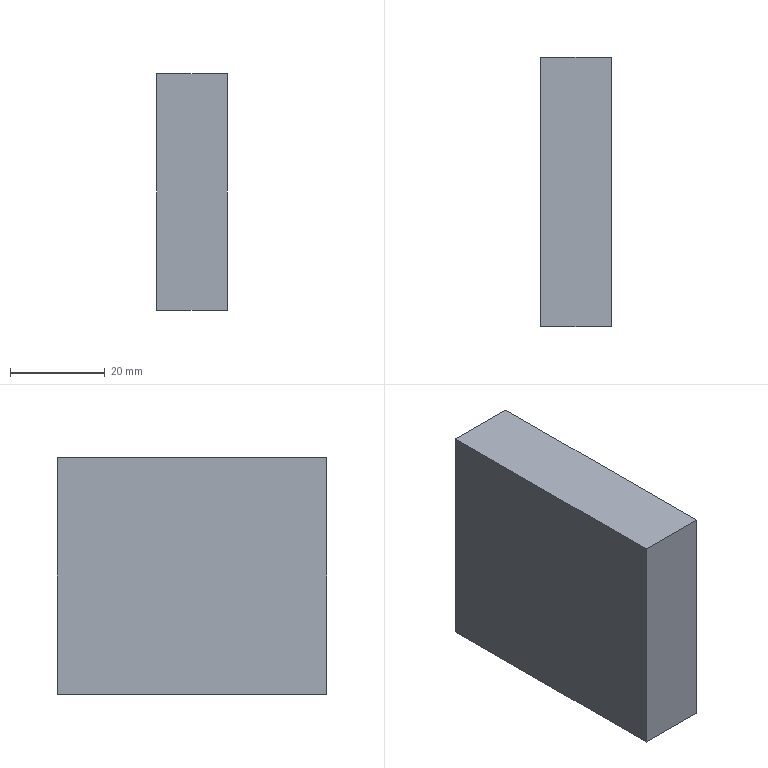Part | STEP file | Vibrator coil left support_default | 1 solid | 18 faces | box 15 x 57 x 50 mm | volume 41837 mm3 | cylinder 6 | cone 6 | plane 6 | commonest cylinder face diameters 5 x6
STEP:
#1=CARTESIAN_POINT('',(0.,0.,0.));
#2=DIRECTION('',(0.,0.,1.));
#3=DIRECTION('',(1.,0.,0.));
#4=AXIS2_PLACEMENT_3D('',#1,#2,#3);
#5=CARTESIAN_POINT('',(-2.5,-17.5,-10.));
#6=VERTEX_POINT('',#5);
#7=CARTESIAN_POINT('',(-2.5,-17.5,-25.));
#8=VERTEX_POINT('',#7);
#9=CARTESIAN_POINT('',(-2.5,-17.5,-25.));
#10=DIRECTION('',(0.,0.,-1.));
#11=VECTOR('',#10,1.);
#12=LINE('',#9,#11);
#13=CARTESIAN_POINT('',(0.,-17.5,-25.));
#14=DIRECTION('',(0.,0.,-1.));
#15=DIRECTION('',(-1.,0.,0.));
#16=AXIS2_PLACEMENT_3D('',#13,#14,#15);
#17=CYLINDRICAL_SURFACE('',#16,2.5);
#18=CARTESIAN_POINT('',(6.283,0.));
#19=DIRECTION('',(0.,1.));
#20=VECTOR('',#19,1.);
#21=LINE('',#18,#20);
#22=(GEOMETRIC_REPRESENTATION_CONTEXT(2)PARAMETRIC_REPRESENTATION_CONTEXT()REPRESENTATION_CONTEXT('',''));
#23=DEFINITIONAL_REPRESENTATION('',(#21),#22);
#24=PCURVE('',#17,#23);
#25=CARTESIAN_POINT('',(0.,-17.5,-25.));
#26=DIRECTION('',(0.,0.,-1.));
#27=DIRECTION('',(-1.,0.,0.));
#28=AXIS2_PLACEMENT_3D('',#25,#26,#27);
#29=CYLINDRICAL_SURFACE('',#28,2.5);
#30=CARTESIAN_POINT('',(0.,0.));
#31=DIRECTION('',(0.,1.));
#32=VECTOR('',#31,1.);
#33=LINE('',#30,#32);
#34=(GEOMETRIC_REPRESENTATION_CONTEXT(2)PARAMETRIC_REPRESENTATION_CONTEXT()REPRESENTATION_CONTEXT('',''));
#35=DEFINITIONAL_REPRESENTATION('',(#33),#34);
#36=PCURVE('',#29,#35);
#37=SURFACE_CURVE('',#12,(#24,#36),.PCURVE_S1.);
#38=EDGE_CURVE('',#6,#8,#37,.T.);
#39=ORIENTED_EDGE('',*,*,#38,.T.);
#40=CARTESIAN_POINT('',(2.5,-17.5,-25.));
#41=VERTEX_POINT('',#40);
#42=CARTESIAN_POINT('',(0.,-17.5,-25.));
#43=DIRECTION('',(0.,0.,-1.));
#44=DIRECTION('',(-1.,0.,0.));
#45=AXIS2_PLACEMENT_3D('',#42,#43,#44);
#46=CIRCLE('',#45,2.5);
#47=CARTESIAN_POINT('',(0.,0.));
#48=DIRECTION('',(1.,0.));
#49=VECTOR('',#48,1.);
#50=LINE('',#47,#49);
#51=(GEOMETRIC_REPRESENTATION_CONTEXT(2)PARAMETRIC_REPRESENTATION_CONTEXT()REPRESENTATION_CONTEXT('',''));
#52=DEFINITIONAL_REPRESENTATION('',(#50),#51);
#53=PCURVE('',#17,#52);
#54=CARTESIAN_POINT('',(0.,0.,-25.));
#55=DIRECTION('',(0.,0.,1.));
#56=DIRECTION('',(1.,0.,0.));
#57=AXIS2_PLACEMENT_3D('',#54,#55,#56);
#58=PLANE('',#57);
#59=CARTESIAN_POINT('',(-2.5,-17.5));
#60=CARTESIAN_POINT('',(-2.5,-13.17));
#61=CARTESIAN_POINT('',(1.25,-15.335));
#62=CARTESIAN_POINT('',(5.,-17.5));
#63=CARTESIAN_POINT('',(1.25,-19.665));
#64=CARTESIAN_POINT('',(-2.5,-21.83));
#65=CARTESIAN_POINT('',(-2.5,-17.5));
#66=(BOUNDED_CURVE()B_SPLINE_CURVE(2,(#59,#60,#61,#62,#63,#64,#65),.UNSPECIFIED.,.T.,.F.)B_SPLINE_CURVE_WITH_KNOTS((1,2,2,2,2,1),(-2.094,0.,2.094,4.189,6.283,8.378),.UNSPECIFIED.)CURVE()GEOMETRIC_REPRESENTATION_ITEM()RATIONAL_B_SPLINE_CURVE((1.,0.5,1.,0.5,1.,0.5,1.))REPRESENTATION_ITEM(''));
#67=(GEOMETRIC_REPRESENTATION_CONTEXT(2)PARAMETRIC_REPRESENTATION_CONTEXT()REPRESENTATION_CONTEXT('',''));
#68=DEFINITIONAL_REPRESENTATION('',(#66),#67);
#69=PCURVE('',#58,#68);
#70=SURFACE_CURVE('',#46,(#53,#69),.PCURVE_S1.);
#71=EDGE_CURVE('',#41,#8,#70,.T.);
#72=ORIENTED_EDGE('',*,*,#71,.F.);
#73=CARTESIAN_POINT('',(2.5,-17.5,-10.));
#74=VERTEX_POINT('',#73);
#75=CARTESIAN_POINT('',(2.5,-17.5,-25.));
#76=DIRECTION('',(0.,0.,-1.));
#77=VECTOR('',#76,1.);
#78=LINE('',#75,#77);
#79=CARTESIAN_POINT('',(3.142,0.));
#80=DIRECTION('',(0.,1.));
#81=VECTOR('',#80,1.);
#82=LINE('',#79,#81);
#83=(GEOMETRIC_REPRESENTATION_CONTEXT(2)PARAMETRIC_REPRESENTATION_CONTEXT()REPRESENTATION_CONTEXT('',''));
#84=DEFINITIONAL_REPRESENTATION('',(#82),#83);
#85=PCURVE('',#17,#84);
#86=CARTESIAN_POINT('',(3.142,0.));
#87=DIRECTION('',(0.,1.));
#88=VECTOR('',#87,1.);
#89=LINE('',#86,#88);
#90=(GEOMETRIC_REPRESENTATION_CONTEXT(2)PARAMETRIC_REPRESENTATION_CONTEXT()REPRESENTATION_CONTEXT('',''));
#91=DEFINITIONAL_REPRESENTATION('',(#89),#90);
#92=PCURVE('',#29,#91);
#93=SURFACE_CURVE('',#78,(#85,#92),.PCURVE_S1.);
#94=EDGE_CURVE('',#74,#41,#93,.T.);
#95=ORIENTED_EDGE('',*,*,#94,.F.);
#96=CARTESIAN_POINT('',(0.,-17.5,-10.));
#97=DIRECTION('',(0.,0.,-1.));
#98=DIRECTION('',(-1.,0.,0.));
#99=AXIS2_PLACEMENT_3D('',#96,#97,#98);
#100=CIRCLE('',#99,2.5);
#101=CARTESIAN_POINT('',(0.,-15.));
#102=DIRECTION('',(1.,0.));
#103=VECTOR('',#102,1.);
#104=LINE('',#101,#103);
#105=(GEOMETRIC_REPRESENTATION_CONTEXT(2)PARAMETRIC_REPRESENTATION_CONTEXT()REPRESENTATION_CONTEXT('',''));
#106=DEFINITIONAL_REPRESENTATION('',(#104),#105);
#107=PCURVE('',#17,#106);
#108=CARTESIAN_POINT('',(0.,-17.5,-10.));
#109=DIRECTION('',(0.,0.,-1.));
#110=DIRECTION('',(-1.,0.,0.));
#111=AXIS2_PLACEMENT_3D('',#108,#109,#110);
#112=CONICAL_SURFACE('',#111,2.5,1.03);
#113=CARTESIAN_POINT('',(0.,0.));
#114=DIRECTION('',(1.,0.));
#115=VECTOR('',#114,1.);
#116=LINE('',#113,#115);
#117=(GEOMETRIC_REPRESENTATION_CONTEXT(2)PARAMETRIC_REPRESENTATION_CONTEXT()REPRESENTATION_CONTEXT('',''));
#118=DEFINITIONAL_REPRESENTATION('',(#116),#117);
#119=PCURVE('',#112,#118);
#120=SURFACE_CURVE('',#100,(#107,#119),.PCURVE_S1.);
#121=EDGE_CURVE('',#74,#6,#120,.T.);
#122=ORIENTED_EDGE('',*,*,#121,.T.);
#123=EDGE_LOOP('',(#39,#72,#95,#122));
#124=FACE_BOUND('',#123,.F.);
#125=ADVANCED_FACE('',(#124),#17,.F.);
#126=ORIENTED_EDGE('',*,*,#121,.F.);
#127=CARTESIAN_POINT('',(0.,-17.5,-8.498));
#128=VERTEX_POINT('',#127);
#129=CARTESIAN_POINT('',(2.5,-17.5,-10.));
#130=DIRECTION('',(0.8572,0.,-0.515));
#131=VECTOR('',#130,1.);
#132=LINE('',#129,#131);
#133=CARTESIAN_POINT('',(3.142,0.));
#134=DIRECTION('',(0.,1.));
#135=VECTOR('',#134,1.);
#136=LINE('',#133,#135);
#137=(GEOMETRIC_REPRESENTATION_CONTEXT(2)PARAMETRIC_REPRESENTATION_CONTEXT()REPRESENTATION_CONTEXT('',''));
#138=DEFINITIONAL_REPRESENTATION('',(#136),#137);
#139=PCURVE('',#112,#138);
#140=CARTESIAN_POINT('',(0.,-17.5,-10.));
#141=DIRECTION('',(0.,0.,-1.));
#142=DIRECTION('',(-1.,0.,0.));
#143=AXIS2_PLACEMENT_3D('',#140,#141,#142);
#144=CONICAL_SURFACE('',#143,2.5,1.03);
#145=CARTESIAN_POINT('',(3.142,0.));
#146=DIRECTION('',(0.,1.));
#147=VECTOR('',#146,1.);
#148=LINE('',#145,#147);
#149=(GEOMETRIC_REPRESENTATION_CONTEXT(2)PARAMETRIC_REPRESENTATION_CONTEXT()REPRESENTATION_CONTEXT('',''));
#150=DEFINITIONAL_REPRESENTATION('',(#148),#149);
#151=PCURVE('',#144,#150);
#152=SURFACE_CURVE('',#132,(#139,#151),.PCURVE_S1.);
#153=EDGE_CURVE('',#128,#74,#152,.T.);
#154=ORIENTED_EDGE('',*,*,#153,.F.);
#155=CARTESIAN_POINT('',(-2.5,-17.5,-10.));
#156=DIRECTION('',(-0.8572,0.,-0.515));
#157=VECTOR('',#156,1.);
#158=LINE('',#155,#157);
#159=CARTESIAN_POINT('',(6.283,0.));
#160=DIRECTION('',(0.,1.));
#161=VECTOR('',#160,1.);
#162=LINE('',#159,#161);
#163=(GEOMETRIC_REPRESENTATION_CONTEXT(2)PARAMETRIC_REPRESENTATION_CONTEXT()REPRESENTATION_CONTEXT('',''));
#164=DEFINITIONAL_REPRESENTATION('',(#162),#163);
#165=PCURVE('',#112,#164);
#166=CARTESIAN_POINT('',(0.,0.));
#167=DIRECTION('',(0.,1.));
#168=VECTOR('',#167,1.);
#169=LINE('',#166,#168);
#170=(GEOMETRIC_REPRESENTATION_CONTEXT(2)PARAMETRIC_REPRESENTATION_CONTEXT()REPRESENTATION_CONTEXT('',''));
#171=DEFINITIONAL_REPRESENTATION('',(#169),#170);
#172=PCURVE('',#144,#171);
#173=SURFACE_CURVE('',#158,(#165,#172),.PCURVE_S1.);
#174=EDGE_CURVE('',#128,#6,#173,.T.);
#175=ORIENTED_EDGE('',*,*,#174,.T.);
#176=EDGE_LOOP('',(#126,#154,#175));
#177=FACE_BOUND('',#176,.F.);
#178=ADVANCED_FACE('',(#177),#112,.F.);
#179=CARTESIAN_POINT('',(-2.5,17.5,-10.));
#180=VERTEX_POINT('',#179);
#181=CARTESIAN_POINT('',(-2.5,17.5,-25.));
#182=VERTEX_POINT('',#181);
#183=CARTESIAN_POINT('',(-2.5,17.5,-25.));
#184=DIRECTION('',(0.,0.,-1.));
#185=VECTOR('',#184,1.);
#186=LINE('',#183,#185);
#187=CARTESIAN_POINT('',(0.,17.5,-25.));
#188=DIRECTION('',(0.,0.,-1.));
#189=DIRECTION('',(-1.,0.,0.));
#190=AXIS2_PLACEMENT_3D('',#187,#188,#189);
#191=CYLINDRICAL_SURFACE('',#190,2.5);
#192=CARTESIAN_POINT('',(6.283,0.));
#193=DIRECTION('',(0.,1.));
#194=VECTOR('',#193,1.);
#195=LINE('',#192,#194);
#196=(GEOMETRIC_REPRESENTATION_CONTEXT(2)PARAMETRIC_REPRESENTATION_CONTEXT()REPRESENTATION_CONTEXT('',''));
#197=DEFINITIONAL_REPRESENTATION('',(#195),#196);
#198=PCURVE('',#191,#197);
#199=CARTESIAN_POINT('',(0.,17.5,-25.));
#200=DIRECTION('',(0.,0.,-1.));
#201=DIRECTION('',(-1.,0.,0.));
#202=AXIS2_PLACEMENT_3D('',#199,#200,#201);
#203=CYLINDRICAL_SURFACE('',#202,2.5);
#204=CARTESIAN_POINT('',(0.,0.));
#205=DIRECTION('',(0.,1.));
#206=VECTOR('',#205,1.);
#207=LINE('',#204,#206);
#208=(GEOMETRIC_REPRESENTATION_CONTEXT(2)PARAMETRIC_REPRESENTATION_CONTEXT()REPRESENTATION_CONTEXT('',''));
#209=DEFINITIONAL_REPRESENTATION('',(#207),#208);
#210=PCURVE('',#203,#209);
#211=SURFACE_CURVE('',#186,(#198,#210),.PCURVE_S1.);
#212=EDGE_CURVE('',#180,#182,#211,.T.);
#213=ORIENTED_EDGE('',*,*,#212,.T.);
#214=CARTESIAN_POINT('',(2.5,17.5,-25.));
#215=VERTEX_POINT('',#214);
#216=CARTESIAN_POINT('',(0.,17.5,-25.));
#217=DIRECTION('',(0.,0.,-1.));
#218=DIRECTION('',(-1.,0.,0.));
#219=AXIS2_PLACEMENT_3D('',#216,#217,#218);
#220=CIRCLE('',#219,2.5);
#221=CARTESIAN_POINT('',(0.,0.));
#222=DIRECTION('',(1.,0.));
#223=VECTOR('',#222,1.);
#224=LINE('',#221,#223);
#225=(GEOMETRIC_REPRESENTATION_CONTEXT(2)PARAMETRIC_REPRESENTATION_CONTEXT()REPRESENTATION_CONTEXT('',''));
#226=DEFINITIONAL_REPRESENTATION('',(#224),#225);
#227=PCURVE('',#191,#226);
#228=CARTESIAN_POINT('',(-2.5,17.5));
#229=CARTESIAN_POINT('',(-2.5,21.83));
#230=CARTESIAN_POINT('',(1.25,19.665));
#231=CARTESIAN_POINT('',(5.,17.5));
#232=CARTESIAN_POINT('',(1.25,15.335));
#233=CARTESIAN_POINT('',(-2.5,13.17));
#234=CARTESIAN_POINT('',(-2.5,17.5));
#235=(BOUNDED_CURVE()B_SPLINE_CURVE(2,(#228,#229,#230,#231,#232,#233,#234),.UNSPECIFIED.,.T.,.F.)B_SPLINE_CURVE_WITH_KNOTS((1,2,2,2,2,1),(-2.094,0.,2.094,4.189,6.283,8.378),.UNSPECIFIED.)CURVE()GEOMETRIC_REPRESENTATION_ITEM()RATIONAL_B_SPLINE_CURVE((1.,0.5,1.,0.5,1.,0.5,1.))REPRESENTATION_ITEM(''));
#236=(GEOMETRIC_REPRESENTATION_CONTEXT(2)PARAMETRIC_REPRESENTATION_CONTEXT()REPRESENTATION_CONTEXT('',''));
#237=DEFINITIONAL_REPRESENTATION('',(#235),#236);
#238=PCURVE('',#58,#237);
#239=SURFACE_CURVE('',#220,(#227,#238),.PCURVE_S1.);
#240=EDGE_CURVE('',#215,#182,#239,.T.);
#241=ORIENTED_EDGE('',*,*,#240,.F.);
#242=CARTESIAN_POINT('',(2.5,17.5,-10.));
#243=VERTEX_POINT('',#242);
#244=CARTESIAN_POINT('',(2.5,17.5,-25.));
#245=DIRECTION('',(0.,0.,-1.));
#246=VECTOR('',#245,1.);
#247=LINE('',#244,#246);
#248=CARTESIAN_POINT('',(3.142,0.));
#249=DIRECTION('',(0.,1.));
#250=VECTOR('',#249,1.);
#251=LINE('',#248,#250);
#252=(GEOMETRIC_REPRESENTATION_CONTEXT(2)PARAMETRIC_REPRESENTATION_CONTEXT()REPRESENTATION_CONTEXT('',''));
#253=DEFINITIONAL_REPRESENTATION('',(#251),#252);
#254=PCURVE('',#191,#253);
#255=CARTESIAN_POINT('',(3.142,0.));
#256=DIRECTION('',(0.,1.));
#257=VECTOR('',#256,1.);
#258=LINE('',#255,#257);
#259=(GEOMETRIC_REPRESENTATION_CONTEXT(2)PARAMETRIC_REPRESENTATION_CONTEXT()REPRESENTATION_CONTEXT('',''));
#260=DEFINITIONAL_REPRESENTATION('',(#258),#259);
#261=PCURVE('',#203,#260);
#262=SURFACE_CURVE('',#247,(#254,#261),.PCURVE_S1.);
#263=EDGE_CURVE('',#243,#215,#262,.T.);
#264=ORIENTED_EDGE('',*,*,#263,.F.);
#265=CARTESIAN_POINT('',(0.,17.5,-10.));
#266=DIRECTION('',(0.,0.,-1.));
#267=DIRECTION('',(-1.,0.,0.));
#268=AXIS2_PLACEMENT_3D('',#265,#266,#267);
#269=CIRCLE('',#268,2.5);
#270=CARTESIAN_POINT('',(0.,-15.));
#271=DIRECTION('',(1.,0.));
#272=VECTOR('',#271,1.);
#273=LINE('',#270,#272);
#274=(GEOMETRIC_REPRESENTATION_CONTEXT(2)PARAMETRIC_REPRESENTATION_CONTEXT()REPRESENTATION_CONTEXT('',''));
#275=DEFINITIONAL_REPRESENTATION('',(#273),#274);
#276=PCURVE('',#191,#275);
#277=CARTESIAN_POINT('',(0.,17.5,-10.));
#278=DIRECTION('',(0.,0.,-1.));
#279=DIRECTION('',(-1.,0.,0.));
#280=AXIS2_PLACEMENT_3D('',#277,#278,#279);
#281=CONICAL_SURFACE('',#280,2.5,1.03);
#282=CARTESIAN_POINT('',(0.,0.));
#283=DIRECTION('',(1.,0.));
#284=VECTOR('',#283,1.);
#285=LINE('',#282,#284);
#286=(GEOMETRIC_REPRESENTATION_CONTEXT(2)PARAMETRIC_REPRESENTATION_CONTEXT()REPRESENTATION_CONTEXT('',''));
#287=DEFINITIONAL_REPRESENTATION('',(#285),#286);
#288=PCURVE('',#281,#287);
#289=SURFACE_CURVE('',#269,(#276,#288),.PCURVE_S1.);
#290=EDGE_CURVE('',#243,#180,#289,.T.);
#291=ORIENTED_EDGE('',*,*,#290,.T.);
#292=EDGE_LOOP('',(#213,#241,#264,#291));
#293=FACE_BOUND('',#292,.F.);
#294=ADVANCED_FACE('',(#293),#191,.F.);
#295=ORIENTED_EDGE('',*,*,#290,.F.);
#296=CARTESIAN_POINT('',(0.,17.5,-8.498));
#297=VERTEX_POINT('',#296);
#298=CARTESIAN_POINT('',(2.5,17.5,-10.));
#299=DIRECTION('',(0.8572,0.,-0.515));
#300=VECTOR('',#299,1.);
#301=LINE('',#298,#300);
#302=CARTESIAN_POINT('',(3.142,0.));
#303=DIRECTION('',(0.,1.));
#304=VECTOR('',#303,1.);
#305=LINE('',#302,#304);
#306=(GEOMETRIC_REPRESENTATION_CONTEXT(2)PARAMETRIC_REPRESENTATION_CONTEXT()REPRESENTATION_CONTEXT('',''));
#307=DEFINITIONAL_REPRESENTATION('',(#305),#306);
#308=PCURVE('',#281,#307);
#309=CARTESIAN_POINT('',(0.,17.5,-10.));
#310=DIRECTION('',(0.,0.,-1.));
#311=DIRECTION('',(-1.,0.,0.));
#312=AXIS2_PLACEMENT_3D('',#309,#310,#311);
#313=CONICAL_SURFACE('',#312,2.5,1.03);
#314=CARTESIAN_POINT('',(3.142,0.));
#315=DIRECTION('',(0.,1.));
#316=VECTOR('',#315,1.);
#317=LINE('',#314,#316);
#318=(GEOMETRIC_REPRESENTATION_CONTEXT(2)PARAMETRIC_REPRESENTATION_CONTEXT()REPRESENTATION_CONTEXT('',''));
#319=DEFINITIONAL_REPRESENTATION('',(#317),#318);
#320=PCURVE('',#313,#319);
#321=SURFACE_CURVE('',#301,(#308,#320),.PCURVE_S1.);
#322=EDGE_CURVE('',#297,#243,#321,.T.);
#323=ORIENTED_EDGE('',*,*,#322,.F.);
#324=CARTESIAN_POINT('',(-2.5,17.5,-10.));
#325=DIRECTION('',(-0.8572,0.,-0.515));
#326=VECTOR('',#325,1.);
#327=LINE('',#324,#326);
#328=CARTESIAN_POINT('',(6.283,0.));
#329=DIRECTION('',(0.,1.));
#330=VECTOR('',#329,1.);
#331=LINE('',#328,#330);
#332=(GEOMETRIC_REPRESENTATION_CONTEXT(2)PARAMETRIC_REPRESENTATION_CONTEXT()REPRESENTATION_CONTEXT('',''));
#333=DEFINITIONAL_REPRESENTATION('',(#331),#332);
#334=PCURVE('',#281,#333);
#335=CARTESIAN_POINT('',(0.,0.));
#336=DIRECTION('',(0.,1.));
#337=VECTOR('',#336,1.);
#338=LINE('',#335,#337);
#339=(GEOMETRIC_REPRESENTATION_CONTEXT(2)PARAMETRIC_REPRESENTATION_CONTEXT()REPRESENTATION_CONTEXT('',''));
#340=DEFINITIONAL_REPRESENTATION('',(#338),#339);
#341=PCURVE('',#313,#340);
#342=SURFACE_CURVE('',#327,(#334,#341),.PCURVE_S1.);
#343=EDGE_CURVE('',#297,#180,#342,.T.);
#344=ORIENTED_EDGE('',*,*,#343,.T.);
#345=EDGE_LOOP('',(#295,#323,#344));
#346=FACE_BOUND('',#345,.F.);
#347=ADVANCED_FACE('',(#346),#281,.F.);
#348=CARTESIAN_POINT('',(-2.5,0.,-10.));
#349=VERTEX_POINT('',#348);
#350=CARTESIAN_POINT('',(-2.5,0.,-25.));
#351=VERTEX_POINT('',#350);
#352=CARTESIAN_POINT('',(-2.5,0.,-25.));
#353=DIRECTION('',(0.,0.,-1.));
#354=VECTOR('',#353,1.);
#355=LINE('',#352,#354);
#356=CARTESIAN_POINT('',(0.,0.,-25.));
#357=DIRECTION('',(0.,0.,-1.));
#358=DIRECTION('',(-1.,0.,0.));
#359=AXIS2_PLACEMENT_3D('',#356,#357,#358);
#360=CYLINDRICAL_SURFACE('',#359,2.5);
#361=CARTESIAN_POINT('',(6.283,0.));
#362=DIRECTION('',(0.,1.));
#363=VECTOR('',#362,1.);
#364=LINE('',#361,#363);
#365=(GEOMETRIC_REPRESENTATION_CONTEXT(2)PARAMETRIC_REPRESENTATION_CONTEXT()REPRESENTATION_CONTEXT('',''));
#366=DEFINITIONAL_REPRESENTATION('',(#364),#365);
#367=PCURVE('',#360,#366);
#368=CARTESIAN_POINT('',(0.,0.,-25.));
#369=DIRECTION('',(0.,0.,-1.));
#370=DIRECTION('',(-1.,0.,0.));
#371=AXIS2_PLACEMENT_3D('',#368,#369,#370);
#372=CYLINDRICAL_SURFACE('',#371,2.5);
#373=CARTESIAN_POINT('',(0.,0.));
#374=DIRECTION('',(0.,1.));
#375=VECTOR('',#374,1.);
#376=LINE('',#373,#375);
#377=(GEOMETRIC_REPRESENTATION_CONTEXT(2)PARAMETRIC_REPRESENTATION_CONTEXT()REPRESENTATION_CONTEXT('',''));
#378=DEFINITIONAL_REPRESENTATION('',(#376),#377);
#379=PCURVE('',#372,#378);
#380=SURFACE_CURVE('',#355,(#367,#379),.PCURVE_S1.);
#381=EDGE_CURVE('',#349,#351,#380,.T.);
#382=ORIENTED_EDGE('',*,*,#381,.T.);
#383=CARTESIAN_POINT('',(2.5,0.,-25.));
#384=VERTEX_POINT('',#383);
#385=CARTESIAN_POINT('',(0.,0.,-25.));
#386=DIRECTION('',(0.,0.,-1.));
#387=DIRECTION('',(-1.,0.,0.));
#388=AXIS2_PLACEMENT_3D('',#385,#386,#387);
#389=CIRCLE('',#388,2.5);
#390=CARTESIAN_POINT('',(0.,0.));
#391=DIRECTION('',(1.,0.));
#392=VECTOR('',#391,1.);
#393=LINE('',#390,#392);
#394=(GEOMETRIC_REPRESENTATION_CONTEXT(2)PARAMETRIC_REPRESENTATION_CONTEXT()REPRESENTATION_CONTEXT('',''));
#395=DEFINITIONAL_REPRESENTATION('',(#393),#394);
#396=PCURVE('',#360,#395);
#397=CARTESIAN_POINT('',(-2.5,0.));
#398=CARTESIAN_POINT('',(-2.5,4.33));
#399=CARTESIAN_POINT('',(1.25,2.165));
#400=CARTESIAN_POINT('',(5.,0.));
#401=CARTESIAN_POINT('',(1.25,-2.165));
#402=CARTESIAN_POINT('',(-2.5,-4.33));
#403=CARTESIAN_POINT('',(-2.5,0.));
#404=(BOUNDED_CURVE()B_SPLINE_CURVE(2,(#397,#398,#399,#400,#401,#402,#403),.UNSPECIFIED.,.T.,.F.)B_SPLINE_CURVE_WITH_KNOTS((1,2,2,2,2,1),(-2.094,0.,2.094,4.189,6.283,8.378),.UNSPECIFIED.)CURVE()GEOMETRIC_REPRESENTATION_ITEM()RATIONAL_B_SPLINE_CURVE((1.,0.5,1.,0.5,1.,0.5,1.))REPRESENTATION_ITEM(''));
#405=(GEOMETRIC_REPRESENTATION_CONTEXT(2)PARAMETRIC_REPRESENTATION_CONTEXT()REPRESENTATION_CONTEXT('',''));
#406=DEFINITIONAL_REPRESENTATION('',(#404),#405);
#407=PCURVE('',#58,#406);
#408=SURFACE_CURVE('',#389,(#396,#407),.PCURVE_S1.);
#409=EDGE_CURVE('',#384,#351,#408,.T.);
#410=ORIENTED_EDGE('',*,*,#409,.F.);
#411=CARTESIAN_POINT('',(2.5,0.,-10.));
#412=VERTEX_POINT('',#411);
#413=CARTESIAN_POINT('',(2.5,0.,-25.));
#414=DIRECTION('',(0.,0.,-1.));
#415=VECTOR('',#414,1.);
#416=LINE('',#413,#415);
#417=CARTESIAN_POINT('',(3.142,0.));
#418=DIRECTION('',(0.,1.));
#419=VECTOR('',#418,1.);
#420=LINE('',#417,#419);
#421=(GEOMETRIC_REPRESENTATION_CONTEXT(2)PARAMETRIC_REPRESENTATION_CONTEXT()REPRESENTATION_CONTEXT('',''));
#422=DEFINITIONAL_REPRESENTATION('',(#420),#421);
#423=PCURVE('',#360,#422);
#424=CARTESIAN_POINT('',(3.142,0.));
#425=DIRECTION('',(0.,1.));
#426=VECTOR('',#425,1.);
#427=LINE('',#424,#426);
#428=(GEOMETRIC_REPRESENTATION_CONTEXT(2)PARAMETRIC_REPRESENTATION_CONTEXT()REPRESENTATION_CONTEXT('',''));
#429=DEFINITIONAL_REPRESENTATION('',(#427),#428);
#430=PCURVE('',#372,#429);
#431=SURFACE_CURVE('',#416,(#423,#430),.PCURVE_S1.);
#432=EDGE_CURVE('',#412,#384,#431,.T.);
#433=ORIENTED_EDGE('',*,*,#432,.F.);
#434=CARTESIAN_POINT('',(0.,0.,-10.));
#435=DIRECTION('',(0.,0.,-1.));
#436=DIRECTION('',(-1.,0.,0.));
#437=AXIS2_PLACEMENT_3D('',#434,#435,#436);
#438=CIRCLE('',#437,2.5);
#439=CARTESIAN_POINT('',(0.,-15.));
#440=DIRECTION('',(1.,0.));
#441=VECTOR('',#440,1.);
#442=LINE('',#439,#441);
#443=(GEOMETRIC_REPRESENTATION_CONTEXT(2)PARAMETRIC_REPRESENTATION_CONTEXT()REPRESENTATION_CONTEXT('',''));
#444=DEFINITIONAL_REPRESENTATION('',(#442),#443);
#445=PCURVE('',#360,#444);
#446=CARTESIAN_POINT('',(0.,0.,-10.));
#447=DIRECTION('',(0.,0.,-1.));
#448=DIRECTION('',(-1.,0.,0.));
#449=AXIS2_PLACEMENT_3D('',#446,#447,#448);
#450=CONICAL_SURFACE('',#449,2.5,1.03);
#451=CARTESIAN_POINT('',(0.,0.));
#452=DIRECTION('',(1.,0.));
#453=VECTOR('',#452,1.);
#454=LINE('',#451,#453);
#455=(GEOMETRIC_REPRESENTATION_CONTEXT(2)PARAMETRIC_REPRESENTATION_CONTEXT()REPRESENTATION_CONTEXT('',''));
#456=DEFINITIONAL_REPRESENTATION('',(#454),#455);
#457=PCURVE('',#450,#456);
#458=SURFACE_CURVE('',#438,(#445,#457),.PCURVE_S1.);
#459=EDGE_CURVE('',#412,#349,#458,.T.);
#460=ORIENTED_EDGE('',*,*,#459,.T.);
#461=EDGE_LOOP('',(#382,#410,#433,#460));
#462=FACE_BOUND('',#461,.F.);
#463=ADVANCED_FACE('',(#462),#360,.F.);
#464=ORIENTED_EDGE('',*,*,#459,.F.);
#465=CARTESIAN_POINT('',(0.,0.,-8.498));
#466=VERTEX_POINT('',#465);
#467=CARTESIAN_POINT('',(2.5,0.,-10.));
#468=DIRECTION('',(0.8572,0.,-0.515));
#469=VECTOR('',#468,1.);
#470=LINE('',#467,#469);
#471=CARTESIAN_POINT('',(3.142,0.));
#472=DIRECTION('',(0.,1.));
#473=VECTOR('',#472,1.);
#474=LINE('',#471,#473);
#475=(GEOMETRIC_REPRESENTATION_CONTEXT(2)PARAMETRIC_REPRESENTATION_CONTEXT()REPRESENTATION_CONTEXT('',''));
#476=DEFINITIONAL_REPRESENTATION('',(#474),#475);
#477=PCURVE('',#450,#476);
#478=CARTESIAN_POINT('',(0.,0.,-10.));
#479=DIRECTION('',(0.,0.,-1.));
#480=DIRECTION('',(-1.,0.,0.));
#481=AXIS2_PLACEMENT_3D('',#478,#479,#480);
#482=CONICAL_SURFACE('',#481,2.5,1.03);
#483=CARTESIAN_POINT('',(3.142,0.));
#484=DIRECTION('',(0.,1.));
#485=VECTOR('',#484,1.);
#486=LINE('',#483,#485);
#487=(GEOMETRIC_REPRESENTATION_CONTEXT(2)PARAMETRIC_REPRESENTATION_CONTEXT()REPRESENTATION_CONTEXT('',''));
#488=DEFINITIONAL_REPRESENTATION('',(#486),#487);
#489=PCURVE('',#482,#488);
#490=SURFACE_CURVE('',#470,(#477,#489),.PCURVE_S1.);
#491=EDGE_CURVE('',#466,#412,#490,.T.);
#492=ORIENTED_EDGE('',*,*,#491,.F.);
#493=CARTESIAN_POINT('',(-2.5,0.,-10.));
#494=DIRECTION('',(-0.8572,0.,-0.515));
#495=VECTOR('',#494,1.);
#496=LINE('',#493,#495);
#497=CARTESIAN_POINT('',(6.283,0.));
#498=DIRECTION('',(0.,1.));
#499=VECTOR('',#498,1.);
#500=LINE('',#497,#499);
#501=(GEOMETRIC_REPRESENTATION_CONTEXT(2)PARAMETRIC_REPRESENTATION_CONTEXT()REPRESENTATION_CONTEXT('',''));
#502=DEFINITIONAL_REPRESENTATION('',(#500),#501);
#503=PCURVE('',#450,#502);
#504=CARTESIAN_POINT('',(0.,0.));
#505=DIRECTION('',(0.,1.));
#506=VECTOR('',#505,1.);
#507=LINE('',#504,#506);
#508=(GEOMETRIC_REPRESENTATION_CONTEXT(2)PARAMETRIC_REPRESENTATION_CONTEXT()REPRESENTATION_CONTEXT('',''));
#509=DEFINITIONAL_REPRESENTATION('',(#507),#508);
#510=PCURVE('',#482,#509);
#511=SURFACE_CURVE('',#496,(#503,#510),.PCURVE_S1.);
#512=EDGE_CURVE('',#466,#349,#511,.T.);
#513=ORIENTED_EDGE('',*,*,#512,.T.);
#514=EDGE_LOOP('',(#464,#492,#513));
#515=FACE_BOUND('',#514,.F.);
#516=ADVANCED_FACE('',(#515),#450,.F.);
#517=CARTESIAN_POINT('',(-7.5,28.5,-25.));
#518=VERTEX_POINT('',#517);
#519=CARTESIAN_POINT('',(-7.5,-28.5,-25.));
#520=VERTEX_POINT('',#519);
#521=CARTESIAN_POINT('',(-7.5,-28.5,-25.));
#522=DIRECTION('',(0.,-1.,0.));
#523=VECTOR('',#522,1.);
#524=LINE('',#521,#523);
#525=CARTESIAN_POINT('',(-7.5,-28.5,25.));
#526=DIRECTION('',(1.,0.,0.));
#527=DIRECTION('',(0.,0.,-1.));
#528=AXIS2_PLACEMENT_3D('',#525,#526,#527);
#529=PLANE('',#528);
#530=CARTESIAN_POINT('',(50.,0.));
#531=DIRECTION('',(0.,-1.));
#532=VECTOR('',#531,1.);
#533=LINE('',#530,#532);
#534=(GEOMETRIC_REPRESENTATION_CONTEXT(2)PARAMETRIC_REPRESENTATION_CONTEXT()REPRESENTATION_CONTEXT('',''));
#535=DEFINITIONAL_REPRESENTATION('',(#533),#534);
#536=PCURVE('',#529,#535);
#537=CARTESIAN_POINT('',(-7.5,-28.5));
#538=DIRECTION('',(0.,-1.));
#539=VECTOR('',#538,1.);
#540=LINE('',#537,#539);
#541=(GEOMETRIC_REPRESENTATION_CONTEXT(2)PARAMETRIC_REPRESENTATION_CONTEXT()REPRESENTATION_CONTEXT('',''));
#542=DEFINITIONAL_REPRESENTATION('',(#540),#541);
#543=PCURVE('',#58,#542);
#544=SURFACE_CURVE('',#524,(#536,#543),.PCURVE_S1.);
#545=EDGE_CURVE('',#518,#520,#544,.T.);
#546=ORIENTED_EDGE('',*,*,#545,.T.);
#547=CARTESIAN_POINT('',(-7.5,-28.5,25.));
#548=VERTEX_POINT('',#547);
#549=CARTESIAN_POINT('',(-7.5,-28.5,25.));
#550=DIRECTION('',(0.,0.,-1.));
#551=VECTOR('',#550,1.);
#552=LINE('',#549,#551);
#553=CARTESIAN_POINT('',(0.,0.));
#554=DIRECTION('',(1.,0.));
#555=VECTOR('',#554,1.);
#556=LINE('',#553,#555);
#557=(GEOMETRIC_REPRESENTATION_CONTEXT(2)PARAMETRIC_REPRESENTATION_CONTEXT()REPRESENTATION_CONTEXT('',''));
#558=DEFINITIONAL_REPRESENTATION('',(#556),#557);
#559=PCURVE('',#529,#558);
#560=CARTESIAN_POINT('',(7.5,-28.5,25.));
#561=DIRECTION('',(0.,1.,0.));
#562=DIRECTION('',(0.,0.,1.));
#563=AXIS2_PLACEMENT_3D('',#560,#561,#562);
#564=PLANE('',#563);
#565=CARTESIAN_POINT('',(0.,-15.));
#566=DIRECTION('',(-1.,0.));
#567=VECTOR('',#566,1.);
#568=LINE('',#565,#567);
#569=(GEOMETRIC_REPRESENTATION_CONTEXT(2)PARAMETRIC_REPRESENTATION_CONTEXT()REPRESENTATION_CONTEXT('',''));
#570=DEFINITIONAL_REPRESENTATION('',(#568),#569);
#571=PCURVE('',#564,#570);
#572=SURFACE_CURVE('',#552,(#559,#571),.PCURVE_S1.);
#573=EDGE_CURVE('',#548,#520,#572,.T.);
#574=ORIENTED_EDGE('',*,*,#573,.F.);
#575=CARTESIAN_POINT('',(-7.5,28.5,25.));
#576=VERTEX_POINT('',#575);
#577=CARTESIAN_POINT('',(-7.5,-28.5,25.));
#578=DIRECTION('',(0.,-1.,0.));
#579=VECTOR('',#578,1.);
#580=LINE('',#577,#579);
#581=CARTESIAN_POINT('',(0.,0.));
#582=DIRECTION('',(0.,-1.));
#583=VECTOR('',#582,1.);
#584=LINE('',#581,#583);
#585=(GEOMETRIC_REPRESENTATION_CONTEXT(2)PARAMETRIC_REPRESENTATION_CONTEXT()REPRESENTATION_CONTEXT('',''));
#586=DEFINITIONAL_REPRESENTATION('',(#584),#585);
#587=PCURVE('',#529,#586);
#588=CARTESIAN_POINT('',(0.,0.,25.));
#589=DIRECTION('',(0.,0.,1.));
#590=DIRECTION('',(1.,0.,0.));
#591=AXIS2_PLACEMENT_3D('',#588,#589,#590);
#592=PLANE('',#591);
#593=CARTESIAN_POINT('',(-7.5,-28.5));
#594=DIRECTION('',(0.,-1.));
#595=VECTOR('',#594,1.);
#596=LINE('',#593,#595);
#597=(GEOMETRIC_REPRESENTATION_CONTEXT(2)PARAMETRIC_REPRESENTATION_CONTEXT()REPRESENTATION_CONTEXT('',''));
#598=DEFINITIONAL_REPRESENTATION('',(#596),#597);
#599=PCURVE('',#592,#598);
#600=SURFACE_CURVE('',#580,(#587,#599),.PCURVE_S1.);
#601=EDGE_CURVE('',#576,#548,#600,.T.);
#602=ORIENTED_EDGE('',*,*,#601,.F.);
#603=CARTESIAN_POINT('',(-7.5,28.5,25.));
#604=DIRECTION('',(0.,0.,-1.));
#605=VECTOR('',#604,1.);
#606=LINE('',#603,#605);
#607=CARTESIAN_POINT('',(0.,57.));
#608=DIRECTION('',(1.,0.));
#609=VECTOR('',#608,1.);
#610=LINE('',#607,#609);
#611=(GEOMETRIC_REPRESENTATION_CONTEXT(2)PARAMETRIC_REPRESENTATION_CONTEXT()REPRESENTATION_CONTEXT('',''));
#612=DEFINITIONAL_REPRESENTATION('',(#610),#611);
#613=PCURVE('',#529,#612);
#614=CARTESIAN_POINT('',(7.5,28.5,25.));
#615=DIRECTION('',(0.,-1.,0.));
#616=DIRECTION('',(0.,0.,-1.));
#617=AXIS2_PLACEMENT_3D('',#614,#615,#616);
#618=PLANE('',#617);
#619=CARTESIAN_POINT('',(0.,-15.));
#620=DIRECTION('',(1.,0.));
#621=VECTOR('',#620,1.);
#622=LINE('',#619,#621);
#623=(GEOMETRIC_REPRESENTATION_CONTEXT(2)PARAMETRIC_REPRESENTATION_CONTEXT()REPRESENTATION_CONTEXT('',''));
#624=DEFINITIONAL_REPRESENTATION('',(#622),#623);
#625=PCURVE('',#618,#624);
#626=SURFACE_CURVE('',#606,(#613,#625),.PCURVE_S1.);
#627=EDGE_CURVE('',#576,#518,#626,.T.);
#628=ORIENTED_EDGE('',*,*,#627,.T.);
#629=EDGE_LOOP('',(#546,#574,#602,#628));
#630=FACE_BOUND('',#629,.T.);
#631=ADVANCED_FACE('',(#630),#529,.F.);
#632=CARTESIAN_POINT('',(7.5,-28.5,-25.));
#633=VERTEX_POINT('',#632);
#634=CARTESIAN_POINT('',(7.5,-28.5,-25.));
#635=DIRECTION('',(1.,0.,0.));
#636=VECTOR('',#635,1.);
#637=LINE('',#634,#636);
#638=CARTESIAN_POINT('',(-50.,0.));
#639=DIRECTION('',(0.,1.));
#640=VECTOR('',#639,1.);
#641=LINE('',#638,#640);
#642=(GEOMETRIC_REPRESENTATION_CONTEXT(2)PARAMETRIC_REPRESENTATION_CONTEXT()REPRESENTATION_CONTEXT('',''));
#643=DEFINITIONAL_REPRESENTATION('',(#641),#642);
#644=PCURVE('',#564,#643);
#645=CARTESIAN_POINT('',(7.5,-28.5));
#646=DIRECTION('',(1.,0.));
#647=VECTOR('',#646,1.);
#648=LINE('',#645,#647);
#649=(GEOMETRIC_REPRESENTATION_CONTEXT(2)PARAMETRIC_REPRESENTATION_CONTEXT()REPRESENTATION_CONTEXT('',''));
#650=DEFINITIONAL_REPRESENTATION('',(#648),#649);
#651=PCURVE('',#58,#650);
#652=SURFACE_CURVE('',#637,(#644,#651),.PCURVE_S1.);
#653=EDGE_CURVE('',#520,#633,#652,.T.);
#654=ORIENTED_EDGE('',*,*,#653,.T.);
#655=CARTESIAN_POINT('',(7.5,-28.5,25.));
#656=VERTEX_POINT('',#655);
#657=CARTESIAN_POINT('',(7.5,-28.5,25.));
#658=DIRECTION('',(0.,0.,-1.));
#659=VECTOR('',#658,1.);
#660=LINE('',#657,#659);
#661=CARTESIAN_POINT('',(0.,0.));
#662=DIRECTION('',(-1.,0.));
#663=VECTOR('',#662,1.);
#664=LINE('',#661,#663);
#665=(GEOMETRIC_REPRESENTATION_CONTEXT(2)PARAMETRIC_REPRESENTATION_CONTEXT()REPRESENTATION_CONTEXT('',''));
#666=DEFINITIONAL_REPRESENTATION('',(#664),#665);
#667=PCURVE('',#564,#666);
#668=CARTESIAN_POINT('',(7.5,-28.5,25.));
#669=DIRECTION('',(-1.,0.,0.));
#670=DIRECTION('',(0.,0.,1.));
#671=AXIS2_PLACEMENT_3D('',#668,#669,#670);
#672=PLANE('',#671);
#673=CARTESIAN_POINT('',(0.,0.));
#674=DIRECTION('',(-1.,0.));
#675=VECTOR('',#674,1.);
#676=LINE('',#673,#675);
#677=(GEOMETRIC_REPRESENTATION_CONTEXT(2)PARAMETRIC_REPRESENTATION_CONTEXT()REPRESENTATION_CONTEXT('',''));
#678=DEFINITIONAL_REPRESENTATION('',(#676),#677);
#679=PCURVE('',#672,#678);
#680=SURFACE_CURVE('',#660,(#667,#679),.PCURVE_S1.);
#681=EDGE_CURVE('',#656,#633,#680,.T.);
#682=ORIENTED_EDGE('',*,*,#681,.F.);
#683=CARTESIAN_POINT('',(7.5,-28.5,25.));
#684=DIRECTION('',(1.,0.,0.));
#685=VECTOR('',#684,1.);
#686=LINE('',#683,#685);
#687=CARTESIAN_POINT('',(0.,0.));
#688=DIRECTION('',(0.,1.));
#689=VECTOR('',#688,1.);
#690=LINE('',#687,#689);
#691=(GEOMETRIC_REPRESENTATION_CONTEXT(2)PARAMETRIC_REPRESENTATION_CONTEXT()REPRESENTATION_CONTEXT('',''));
#692=DEFINITIONAL_REPRESENTATION('',(#690),#691);
#693=PCURVE('',#564,#692);
#694=CARTESIAN_POINT('',(7.5,-28.5));
#695=DIRECTION('',(1.,0.));
#696=VECTOR('',#695,1.);
#697=LINE('',#694,#696);
#698=(GEOMETRIC_REPRESENTATION_CONTEXT(2)PARAMETRIC_REPRESENTATION_CONTEXT()REPRESENTATION_CONTEXT('',''));
#699=DEFINITIONAL_REPRESENTATION('',(#697),#698);
#700=PCURVE('',#592,#699);
#701=SURFACE_CURVE('',#686,(#693,#700),.PCURVE_S1.);
#702=EDGE_CURVE('',#548,#656,#701,.T.);
#703=ORIENTED_EDGE('',*,*,#702,.F.);
#704=ORIENTED_EDGE('',*,*,#573,.T.);
#705=EDGE_LOOP('',(#654,#682,#703,#704));
#706=FACE_BOUND('',#705,.T.);
#707=ADVANCED_FACE('',(#706),#564,.F.);
#708=CARTESIAN_POINT('',(7.5,28.5,-25.));
#709=VERTEX_POINT('',#708);
#710=CARTESIAN_POINT('',(7.5,-28.5,-25.));
#711=DIRECTION('',(0.,1.,0.));
#712=VECTOR('',#711,1.);
#713=LINE('',#710,#712);
#714=CARTESIAN_POINT('',(-50.,0.));
#715=DIRECTION('',(0.,1.));
#716=VECTOR('',#715,1.);
#717=LINE('',#714,#716);
#718=(GEOMETRIC_REPRESENTATION_CONTEXT(2)PARAMETRIC_REPRESENTATION_CONTEXT()REPRESENTATION_CONTEXT('',''));
#719=DEFINITIONAL_REPRESENTATION('',(#717),#718);
#720=PCURVE('',#672,#719);
#721=CARTESIAN_POINT('',(7.5,-28.5));
#722=DIRECTION('',(0.,1.));
#723=VECTOR('',#722,1.);
#724=LINE('',#721,#723);
#725=(GEOMETRIC_REPRESENTATION_CONTEXT(2)PARAMETRIC_REPRESENTATION_CONTEXT()REPRESENTATION_CONTEXT('',''));
#726=DEFINITIONAL_REPRESENTATION('',(#724),#725);
#727=PCURVE('',#58,#726);
#728=SURFACE_CURVE('',#713,(#720,#727),.PCURVE_S1.);
#729=EDGE_CURVE('',#633,#709,#728,.T.);
#730=ORIENTED_EDGE('',*,*,#729,.T.);
#731=CARTESIAN_POINT('',(7.5,28.5,25.));
#732=VERTEX_POINT('',#731);
#733=CARTESIAN_POINT('',(7.5,28.5,25.));
#734=DIRECTION('',(0.,0.,-1.));
#735=VECTOR('',#734,1.);
#736=LINE('',#733,#735);
#737=CARTESIAN_POINT('',(0.,57.));
#738=DIRECTION('',(-1.,0.));
#739=VECTOR('',#738,1.);
#740=LINE('',#737,#739);
#741=(GEOMETRIC_REPRESENTATION_CONTEXT(2)PARAMETRIC_REPRESENTATION_CONTEXT()REPRESENTATION_CONTEXT('',''));
#742=DEFINITIONAL_REPRESENTATION('',(#740),#741);
#743=PCURVE('',#672,#742);
#744=CARTESIAN_POINT('',(0.,0.));
#745=DIRECTION('',(1.,0.));
#746=VECTOR('',#745,1.);
#747=LINE('',#744,#746);
#748=(GEOMETRIC_REPRESENTATION_CONTEXT(2)PARAMETRIC_REPRESENTATION_CONTEXT()REPRESENTATION_CONTEXT('',''));
#749=DEFINITIONAL_REPRESENTATION('',(#747),#748);
#750=PCURVE('',#618,#749);
#751=SURFACE_CURVE('',#736,(#743,#750),.PCURVE_S1.);
#752=EDGE_CURVE('',#732,#709,#751,.T.);
#753=ORIENTED_EDGE('',*,*,#752,.F.);
#754=CARTESIAN_POINT('',(7.5,-28.5,25.));
#755=DIRECTION('',(0.,1.,0.));
#756=VECTOR('',#755,1.);
#757=LINE('',#754,#756);
#758=CARTESIAN_POINT('',(0.,0.));
#759=DIRECTION('',(0.,1.));
#760=VECTOR('',#759,1.);
#761=LINE('',#758,#760);
#762=(GEOMETRIC_REPRESENTATION_CONTEXT(2)PARAMETRIC_REPRESENTATION_CONTEXT()REPRESENTATION_CONTEXT('',''));
#763=DEFINITIONAL_REPRESENTATION('',(#761),#762);
#764=PCURVE('',#672,#763);
#765=CARTESIAN_POINT('',(7.5,-28.5));
#766=DIRECTION('',(0.,1.));
#767=VECTOR('',#766,1.);
#768=LINE('',#765,#767);
#769=(GEOMETRIC_REPRESENTATION_CONTEXT(2)PARAMETRIC_REPRESENTATION_CONTEXT()REPRESENTATION_CONTEXT('',''));
#770=DEFINITIONAL_REPRESENTATION('',(#768),#769);
#771=PCURVE('',#592,#770);
#772=SURFACE_CURVE('',#757,(#764,#771),.PCURVE_S1.);
#773=EDGE_CURVE('',#656,#732,#772,.T.);
#774=ORIENTED_EDGE('',*,*,#773,.F.);
#775=ORIENTED_EDGE('',*,*,#681,.T.);
#776=EDGE_LOOP('',(#730,#753,#774,#775));
#777=FACE_BOUND('',#776,.T.);
#778=ADVANCED_FACE('',(#777),#672,.F.);
#779=CARTESIAN_POINT('',(7.5,28.5,-25.));
#780=DIRECTION('',(-1.,0.,0.));
#781=VECTOR('',#780,1.);
#782=LINE('',#779,#781);
#783=CARTESIAN_POINT('',(50.,0.));
#784=DIRECTION('',(0.,-1.));
#785=VECTOR('',#784,1.);
#786=LINE('',#783,#785);
#787=(GEOMETRIC_REPRESENTATION_CONTEXT(2)PARAMETRIC_REPRESENTATION_CONTEXT()REPRESENTATION_CONTEXT('',''));
#788=DEFINITIONAL_REPRESENTATION('',(#786),#787);
#789=PCURVE('',#618,#788);
#790=CARTESIAN_POINT('',(7.5,28.5));
#791=DIRECTION('',(-1.,0.));
#792=VECTOR('',#791,1.);
#793=LINE('',#790,#792);
#794=(GEOMETRIC_REPRESENTATION_CONTEXT(2)PARAMETRIC_REPRESENTATION_CONTEXT()REPRESENTATION_CONTEXT('',''));
#795=DEFINITIONAL_REPRESENTATION('',(#793),#794);
#796=PCURVE('',#58,#795);
#797=SURFACE_CURVE('',#782,(#789,#796),.PCURVE_S1.);
#798=EDGE_CURVE('',#709,#518,#797,.T.);
#799=ORIENTED_EDGE('',*,*,#798,.T.);
#800=ORIENTED_EDGE('',*,*,#627,.F.);
#801=CARTESIAN_POINT('',(7.5,28.5,25.));
#802=DIRECTION('',(-1.,0.,0.));
#803=VECTOR('',#802,1.);
#804=LINE('',#801,#803);
#805=CARTESIAN_POINT('',(0.,0.));
#806=DIRECTION('',(0.,-1.));
#807=VECTOR('',#806,1.);
#808=LINE('',#805,#807);
#809=(GEOMETRIC_REPRESENTATION_CONTEXT(2)PARAMETRIC_REPRESENTATION_CONTEXT()REPRESENTATION_CONTEXT('',''));
#810=DEFINITIONAL_REPRESENTATION('',(#808),#809);
#811=PCURVE('',#618,#810);
#812=CARTESIAN_POINT('',(7.5,28.5));
#813=DIRECTION('',(-1.,0.));
#814=VECTOR('',#813,1.);
#815=LINE('',#812,#814);
#816=(GEOMETRIC_REPRESENTATION_CONTEXT(2)PARAMETRIC_REPRESENTATION_CONTEXT()REPRESENTATION_CONTEXT('',''));
#817=DEFINITIONAL_REPRESENTATION('',(#815),#816);
#818=PCURVE('',#592,#817);
#819=SURFACE_CURVE('',#804,(#811,#818),.PCURVE_S1.);
#820=EDGE_CURVE('',#732,#576,#819,.T.);
#821=ORIENTED_EDGE('',*,*,#820,.F.);
#822=ORIENTED_EDGE('',*,*,#752,.T.);
#823=EDGE_LOOP('',(#799,#800,#821,#822));
#824=FACE_BOUND('',#823,.T.);
#825=ADVANCED_FACE('',(#824),#618,.F.);
#826=ORIENTED_EDGE('',*,*,#601,.T.);
#827=ORIENTED_EDGE('',*,*,#702,.T.);
#828=ORIENTED_EDGE('',*,*,#773,.T.);
#829=ORIENTED_EDGE('',*,*,#820,.T.);
#830=EDGE_LOOP('',(#826,#827,#828,#829));
#831=FACE_BOUND('',#830,.T.);
#832=ADVANCED_FACE('',(#831),#592,.T.);
#833=CARTESIAN_POINT('',(0.,-17.5,-25.));
#834=DIRECTION('',(0.,0.,-1.));
#835=DIRECTION('',(-1.,0.,0.));
#836=AXIS2_PLACEMENT_3D('',#833,#834,#835);
#837=CIRCLE('',#836,2.5);
#838=CARTESIAN_POINT('',(-2.5,-17.5));
#839=CARTESIAN_POINT('',(-2.5,-13.17));
#840=CARTESIAN_POINT('',(1.25,-15.335));
#841=CARTESIAN_POINT('',(5.,-17.5));
#842=CARTESIAN_POINT('',(1.25,-19.665));
#843=CARTESIAN_POINT('',(-2.5,-21.83));
#844=CARTESIAN_POINT('',(-2.5,-17.5));
#845=(BOUNDED_CURVE()B_SPLINE_CURVE(2,(#838,#839,#840,#841,#842,#843,#844),.UNSPECIFIED.,.T.,.F.)B_SPLINE_CURVE_WITH_KNOTS((1,2,2,2,2,1),(-2.094,0.,2.094,4.189,6.283,8.378),.UNSPECIFIED.)CURVE()GEOMETRIC_REPRESENTATION_ITEM()RATIONAL_B_SPLINE_CURVE((1.,0.5,1.,0.5,1.,0.5,1.))REPRESENTATION_ITEM(''));
#846=(GEOMETRIC_REPRESENTATION_CONTEXT(2)PARAMETRIC_REPRESENTATION_CONTEXT()REPRESENTATION_CONTEXT('',''));
#847=DEFINITIONAL_REPRESENTATION('',(#845),#846);
#848=PCURVE('',#58,#847);
#849=CARTESIAN_POINT('',(0.,0.));
#850=DIRECTION('',(1.,0.));
#851=VECTOR('',#850,1.);
#852=LINE('',#849,#851);
#853=(GEOMETRIC_REPRESENTATION_CONTEXT(2)PARAMETRIC_REPRESENTATION_CONTEXT()REPRESENTATION_CONTEXT('',''));
#854=DEFINITIONAL_REPRESENTATION('',(#852),#853);
#855=PCURVE('',#29,#854);
#856=SURFACE_CURVE('',#837,(#848,#855),.PCURVE_S1.);
#857=EDGE_CURVE('',#8,#41,#856,.T.);
#858=ORIENTED_EDGE('',*,*,#857,.F.);
#859=ORIENTED_EDGE('',*,*,#71,.F.);
#860=EDGE_LOOP('',(#858,#859));
#861=FACE_BOUND('',#860,.T.);
#862=CARTESIAN_POINT('',(0.,17.5,-25.));
#863=DIRECTION('',(0.,0.,-1.));
#864=DIRECTION('',(-1.,0.,0.));
#865=AXIS2_PLACEMENT_3D('',#862,#863,#864);
#866=CIRCLE('',#865,2.5);
#867=CARTESIAN_POINT('',(-2.5,17.5));
#868=CARTESIAN_POINT('',(-2.5,21.83));
#869=CARTESIAN_POINT('',(1.25,19.665));
#870=CARTESIAN_POINT('',(5.,17.5));
#871=CARTESIAN_POINT('',(1.25,15.335));
#872=CARTESIAN_POINT('',(-2.5,13.17));
#873=CARTESIAN_POINT('',(-2.5,17.5));
#874=(BOUNDED_CURVE()B_SPLINE_CURVE(2,(#867,#868,#869,#870,#871,#872,#873),.UNSPECIFIED.,.T.,.F.)B_SPLINE_CURVE_WITH_KNOTS((1,2,2,2,2,1),(-2.094,0.,2.094,4.189,6.283,8.378),.UNSPECIFIED.)CURVE()GEOMETRIC_REPRESENTATION_ITEM()RATIONAL_B_SPLINE_CURVE((1.,0.5,1.,0.5,1.,0.5,1.))REPRESENTATION_ITEM(''));
#875=(GEOMETRIC_REPRESENTATION_CONTEXT(2)PARAMETRIC_REPRESENTATION_CONTEXT()REPRESENTATION_CONTEXT('',''));
#876=DEFINITIONAL_REPRESENTATION('',(#874),#875);
#877=PCURVE('',#58,#876);
#878=CARTESIAN_POINT('',(0.,0.));
#879=DIRECTION('',(1.,0.));
#880=VECTOR('',#879,1.);
#881=LINE('',#878,#880);
#882=(GEOMETRIC_REPRESENTATION_CONTEXT(2)PARAMETRIC_REPRESENTATION_CONTEXT()REPRESENTATION_CONTEXT('',''));
#883=DEFINITIONAL_REPRESENTATION('',(#881),#882);
#884=PCURVE('',#203,#883);
#885=SURFACE_CURVE('',#866,(#877,#884),.PCURVE_S1.);
#886=EDGE_CURVE('',#182,#215,#885,.T.);
#887=ORIENTED_EDGE('',*,*,#886,.F.);
#888=ORIENTED_EDGE('',*,*,#240,.F.);
#889=EDGE_LOOP('',(#887,#888));
#890=FACE_BOUND('',#889,.T.);
#891=CARTESIAN_POINT('',(0.,0.,-25.));
#892=DIRECTION('',(0.,0.,-1.));
#893=DIRECTION('',(-1.,0.,0.));
#894=AXIS2_PLACEMENT_3D('',#891,#892,#893);
#895=CIRCLE('',#894,2.5);
#896=CARTESIAN_POINT('',(-2.5,0.));
#897=CARTESIAN_POINT('',(-2.5,4.33));
#898=CARTESIAN_POINT('',(1.25,2.165));
#899=CARTESIAN_POINT('',(5.,0.));
#900=CARTESIAN_POINT('',(1.25,-2.165));
#901=CARTESIAN_POINT('',(-2.5,-4.33));
#902=CARTESIAN_POINT('',(-2.5,0.));
#903=(BOUNDED_CURVE()B_SPLINE_CURVE(2,(#896,#897,#898,#899,#900,#901,#902),.UNSPECIFIED.,.T.,.F.)B_SPLINE_CURVE_WITH_KNOTS((1,2,2,2,2,1),(-2.094,0.,2.094,4.189,6.283,8.378),.UNSPECIFIED.)CURVE()GEOMETRIC_REPRESENTATION_ITEM()RATIONAL_B_SPLINE_CURVE((1.,0.5,1.,0.5,1.,0.5,1.))REPRESENTATION_ITEM(''));
#904=(GEOMETRIC_REPRESENTATION_CONTEXT(2)PARAMETRIC_REPRESENTATION_CONTEXT()REPRESENTATION_CONTEXT('',''));
#905=DEFINITIONAL_REPRESENTATION('',(#903),#904);
#906=PCURVE('',#58,#905);
#907=CARTESIAN_POINT('',(0.,0.));
#908=DIRECTION('',(1.,0.));
#909=VECTOR('',#908,1.);
#910=LINE('',#907,#909);
#911=(GEOMETRIC_REPRESENTATION_CONTEXT(2)PARAMETRIC_REPRESENTATION_CONTEXT()REPRESENTATION_CONTEXT('',''));
#912=DEFINITIONAL_REPRESENTATION('',(#910),#911);
#913=PCURVE('',#372,#912);
#914=SURFACE_CURVE('',#895,(#906,#913),.PCURVE_S1.);
#915=EDGE_CURVE('',#351,#384,#914,.T.);
#916=ORIENTED_EDGE('',*,*,#915,.F.);
#917=ORIENTED_EDGE('',*,*,#409,.F.);
#918=EDGE_LOOP('',(#916,#917));
#919=FACE_BOUND('',#918,.T.);
#920=ORIENTED_EDGE('',*,*,#545,.F.);
#921=ORIENTED_EDGE('',*,*,#798,.F.);
#922=ORIENTED_EDGE('',*,*,#729,.F.);
#923=ORIENTED_EDGE('',*,*,#653,.F.);
#924=EDGE_LOOP('',(#920,#921,#922,#923));
#925=FACE_BOUND('',#924,.T.);
#926=ADVANCED_FACE('',(#861,#890,#919,#925),#58,.F.);
#927=CARTESIAN_POINT('',(0.,0.,-10.));
#928=DIRECTION('',(0.,0.,-1.));
#929=DIRECTION('',(-1.,0.,0.));
#930=AXIS2_PLACEMENT_3D('',#927,#928,#929);
#931=CIRCLE('',#930,2.5);
#932=CARTESIAN_POINT('',(0.,0.));
#933=DIRECTION('',(1.,0.));
#934=VECTOR('',#933,1.);
#935=LINE('',#932,#934);
#936=(GEOMETRIC_REPRESENTATION_CONTEXT(2)PARAMETRIC_REPRESENTATION_CONTEXT()REPRESENTATION_CONTEXT('',''));
#937=DEFINITIONAL_REPRESENTATION('',(#935),#936);
#938=PCURVE('',#482,#937);
#939=CARTESIAN_POINT('',(0.,-15.));
#940=DIRECTION('',(1.,0.));
#941=VECTOR('',#940,1.);
#942=LINE('',#939,#941);
#943=(GEOMETRIC_REPRESENTATION_CONTEXT(2)PARAMETRIC_REPRESENTATION_CONTEXT()REPRESENTATION_CONTEXT('',''));
#944=DEFINITIONAL_REPRESENTATION('',(#942),#943);
#945=PCURVE('',#372,#944);
#946=SURFACE_CURVE('',#931,(#938,#945),.PCURVE_S1.);
#947=EDGE_CURVE('',#349,#412,#946,.T.);
#948=ORIENTED_EDGE('',*,*,#947,.F.);
#949=ORIENTED_EDGE('',*,*,#512,.F.);
#950=ORIENTED_EDGE('',*,*,#491,.T.);
#951=EDGE_LOOP('',(#948,#949,#950));
#952=FACE_BOUND('',#951,.F.);
#953=ADVANCED_FACE('',(#952),#482,.F.);
#954=ORIENTED_EDGE('',*,*,#915,.F.);
#955=ORIENTED_EDGE('',*,*,#381,.F.);
#956=ORIENTED_EDGE('',*,*,#947,.T.);
#957=ORIENTED_EDGE('',*,*,#432,.T.);
#958=EDGE_LOOP('',(#954,#955,#956,#957));
#959=FACE_BOUND('',#958,.F.);
#960=ADVANCED_FACE('',(#959),#372,.F.);
#961=CARTESIAN_POINT('',(0.,17.5,-10.));
#962=DIRECTION('',(0.,0.,-1.));
#963=DIRECTION('',(-1.,0.,0.));
#964=AXIS2_PLACEMENT_3D('',#961,#962,#963);
#965=CIRCLE('',#964,2.5);
#966=CARTESIAN_POINT('',(0.,0.));
#967=DIRECTION('',(1.,0.));
#968=VECTOR('',#967,1.);
#969=LINE('',#966,#968);
#970=(GEOMETRIC_REPRESENTATION_CONTEXT(2)PARAMETRIC_REPRESENTATION_CONTEXT()REPRESENTATION_CONTEXT('',''));
#971=DEFINITIONAL_REPRESENTATION('',(#969),#970);
#972=PCURVE('',#313,#971);
#973=CARTESIAN_POINT('',(0.,-15.));
#974=DIRECTION('',(1.,0.));
#975=VECTOR('',#974,1.);
#976=LINE('',#973,#975);
#977=(GEOMETRIC_REPRESENTATION_CONTEXT(2)PARAMETRIC_REPRESENTATION_CONTEXT()REPRESENTATION_CONTEXT('',''));
#978=DEFINITIONAL_REPRESENTATION('',(#976),#977);
#979=PCURVE('',#203,#978);
#980=SURFACE_CURVE('',#965,(#972,#979),.PCURVE_S1.);
#981=EDGE_CURVE('',#180,#243,#980,.T.);
#982=ORIENTED_EDGE('',*,*,#981,.F.);
#983=ORIENTED_EDGE('',*,*,#343,.F.);
#984=ORIENTED_EDGE('',*,*,#322,.T.);
#985=EDGE_LOOP('',(#982,#983,#984));
#986=FACE_BOUND('',#985,.F.);
#987=ADVANCED_FACE('',(#986),#313,.F.);
#988=ORIENTED_EDGE('',*,*,#886,.F.);
#989=ORIENTED_EDGE('',*,*,#212,.F.);
#990=ORIENTED_EDGE('',*,*,#981,.T.);
#991=ORIENTED_EDGE('',*,*,#263,.T.);
#992=EDGE_LOOP('',(#988,#989,#990,#991));
#993=FACE_BOUND('',#992,.F.);
#994=ADVANCED_FACE('',(#993),#203,.F.);
#995=CARTESIAN_POINT('',(0.,-17.5,-10.));
#996=DIRECTION('',(0.,0.,-1.));
#997=DIRECTION('',(-1.,0.,0.));
#998=AXIS2_PLACEMENT_3D('',#995,#996,#997);
#999=CIRCLE('',#998,2.5);
#1000=CARTESIAN_POINT('',(0.,0.));
#1001=DIRECTION('',(1.,0.));
#1002=VECTOR('',#1001,1.);
#1003=LINE('',#1000,#1002);
#1004=(GEOMETRIC_REPRESENTATION_CONTEXT(2)PARAMETRIC_REPRESENTATION_CONTEXT()REPRESENTATION_CONTEXT('',''));
#1005=DEFINITIONAL_REPRESENTATION('',(#1003),#1004);
#1006=PCURVE('',#144,#1005);
#1007=CARTESIAN_POINT('',(0.,-15.));
#1008=DIRECTION('',(1.,0.));
#1009=VECTOR('',#1008,1.);
#1010=LINE('',#1007,#1009);
#1011=(GEOMETRIC_REPRESENTATION_CONTEXT(2)PARAMETRIC_REPRESENTATION_CONTEXT()REPRESENTATION_CONTEXT('',''));
#1012=DEFINITIONAL_REPRESENTATION('',(#1010),#1011);
#1013=PCURVE('',#29,#1012);
#1014=SURFACE_CURVE('',#999,(#1006,#1013),.PCURVE_S1.);
#1015=EDGE_CURVE('',#6,#74,#1014,.T.);
#1016=ORIENTED_EDGE('',*,*,#1015,.F.);
#1017=ORIENTED_EDGE('',*,*,#174,.F.);
#1018=ORIENTED_EDGE('',*,*,#153,.T.);
#1019=EDGE_LOOP('',(#1016,#1017,#1018));
#1020=FACE_BOUND('',#1019,.F.);
#1021=ADVANCED_FACE('',(#1020),#144,.F.);
#1022=ORIENTED_EDGE('',*,*,#857,.F.);
#1023=ORIENTED_EDGE('',*,*,#38,.F.);
#1024=ORIENTED_EDGE('',*,*,#1015,.T.);
#1025=ORIENTED_EDGE('',*,*,#94,.T.);
#1026=EDGE_LOOP('',(#1022,#1023,#1024,#1025));
#1027=FACE_BOUND('',#1026,.F.);
#1028=ADVANCED_FACE('',(#1027),#29,.F.);
#1029=CLOSED_SHELL('',(#125,#178,#294,#347,#463,#516,#631,#707,#778,#825,#832,#926,#953,#960,#987,#994,#1021,#1028));
#1030=MANIFOLD_SOLID_BREP('',#1029);
#1031=(LENGTH_UNIT()NAMED_UNIT(*)SI_UNIT(.MILLI.,.METRE.));
#1032=UNCERTAINTY_MEASURE_WITH_UNIT(LENGTH_MEASURE(0.0000001),#1031,'','');
#1033=(NAMED_UNIT(*)PLANE_ANGLE_UNIT()SI_UNIT($,.RADIAN.));
#1034=(NAMED_UNIT(*)SI_UNIT($,.STERADIAN.)SOLID_ANGLE_UNIT());
#1035=(GEOMETRIC_REPRESENTATION_CONTEXT(3)GLOBAL_UNCERTAINTY_ASSIGNED_CONTEXT((#1032))GLOBAL_UNIT_ASSIGNED_CONTEXT((#1031,#1033,#1034))REPRESENTATION_CONTEXT('',''));
#1036=ADVANCED_BREP_SHAPE_REPRESENTATION('',(#4,#1030),#1035);